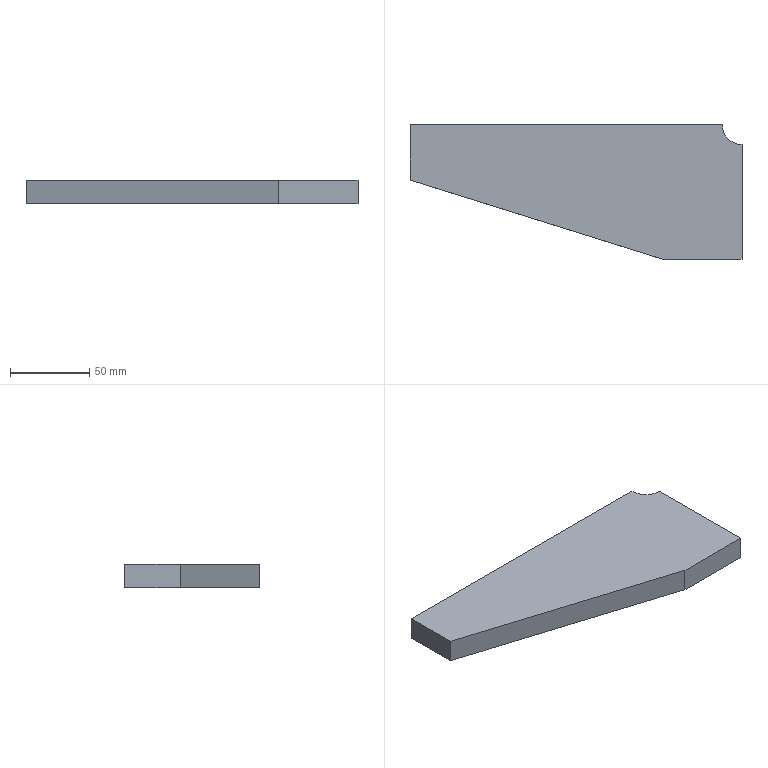Part | STEP file | Input 77 | 1 solid | 8 faces | box 210 x 85 x 15 mm | volume 205909 mm3 | plane 7 | cylinder 1 | commonest cylinder face diameters 25 x1
STEP:
#1=CARTESIAN_POINT('',(0.,0.,0.));
#2=DIRECTION('',(0.,0.,1.));
#3=DIRECTION('',(1.,0.,0.));
#4=AXIS2_PLACEMENT_3D('',#1,#2,#3);
#5=CARTESIAN_POINT('',(4010.,310.,-7.5));
#6=VERTEX_POINT('',#5);
#7=CARTESIAN_POINT('',(3960.,310.,-7.5));
#8=VERTEX_POINT('',#7);
#9=CARTESIAN_POINT('',(3960.,310.,-7.5));
#10=DIRECTION('',(-1.,0.,0.));
#11=VECTOR('',#10,1.);
#12=LINE('',#9,#11);
#13=CARTESIAN_POINT('',(3960.,310.,7.5));
#14=DIRECTION('',(0.,-1.,0.));
#15=DIRECTION('',(-1.,0.,0.));
#16=AXIS2_PLACEMENT_3D('',#13,#14,#15);
#17=PLANE('',#16);
#18=CARTESIAN_POINT('',(0.,15.));
#19=DIRECTION('',(1.,0.));
#20=VECTOR('',#19,1.);
#21=LINE('',#18,#20);
#22=(GEOMETRIC_REPRESENTATION_CONTEXT(2)PARAMETRIC_REPRESENTATION_CONTEXT()REPRESENTATION_CONTEXT('',''));
#23=DEFINITIONAL_REPRESENTATION('',(#21),#22);
#24=PCURVE('',#17,#23);
#25=CARTESIAN_POINT('',(4010.,395.,-7.5));
#26=DIRECTION('',(0.,0.,-1.));
#27=DIRECTION('',(-1.,0.,0.));
#28=AXIS2_PLACEMENT_3D('',#25,#26,#27);
#29=PLANE('',#28);
#30=CARTESIAN_POINT('',(50.,-85.));
#31=DIRECTION('',(1.,0.));
#32=VECTOR('',#31,1.);
#33=LINE('',#30,#32);
#34=(GEOMETRIC_REPRESENTATION_CONTEXT(2)PARAMETRIC_REPRESENTATION_CONTEXT()REPRESENTATION_CONTEXT('',''));
#35=DEFINITIONAL_REPRESENTATION('',(#33),#34);
#36=PCURVE('',#29,#35);
#37=SURFACE_CURVE('',#12,(#24,#36),.PCURVE_S1.);
#38=EDGE_CURVE('',#6,#8,#37,.T.);
#39=ORIENTED_EDGE('',*,*,#38,.F.);
#40=CARTESIAN_POINT('',(4010.,310.,7.5));
#41=VERTEX_POINT('',#40);
#42=CARTESIAN_POINT('',(4010.,310.,7.5));
#43=DIRECTION('',(0.,0.,-1.));
#44=VECTOR('',#43,1.);
#45=LINE('',#42,#44);
#46=CARTESIAN_POINT('',(-50.,0.));
#47=DIRECTION('',(0.,1.));
#48=VECTOR('',#47,1.);
#49=LINE('',#46,#48);
#50=(GEOMETRIC_REPRESENTATION_CONTEXT(2)PARAMETRIC_REPRESENTATION_CONTEXT()REPRESENTATION_CONTEXT('',''));
#51=DEFINITIONAL_REPRESENTATION('',(#49),#50);
#52=PCURVE('',#17,#51);
#53=CARTESIAN_POINT('',(4010.,310.,7.5));
#54=DIRECTION('',(1.,0.,0.));
#55=DIRECTION('',(0.,0.,-1.));
#56=AXIS2_PLACEMENT_3D('',#53,#54,#55);
#57=PLANE('',#56);
#58=CARTESIAN_POINT('',(0.,0.));
#59=DIRECTION('',(1.,0.));
#60=VECTOR('',#59,1.);
#61=LINE('',#58,#60);
#62=(GEOMETRIC_REPRESENTATION_CONTEXT(2)PARAMETRIC_REPRESENTATION_CONTEXT()REPRESENTATION_CONTEXT('',''));
#63=DEFINITIONAL_REPRESENTATION('',(#61),#62);
#64=PCURVE('',#57,#63);
#65=SURFACE_CURVE('',#45,(#52,#64),.PCURVE_S1.);
#66=EDGE_CURVE('',#41,#6,#65,.T.);
#67=ORIENTED_EDGE('',*,*,#66,.F.);
#68=CARTESIAN_POINT('',(3960.,310.,7.5));
#69=VERTEX_POINT('',#68);
#70=CARTESIAN_POINT('',(3960.,310.,7.5));
#71=DIRECTION('',(-1.,0.,0.));
#72=VECTOR('',#71,1.);
#73=LINE('',#70,#72);
#74=CARTESIAN_POINT('',(0.,0.));
#75=DIRECTION('',(1.,0.));
#76=VECTOR('',#75,1.);
#77=LINE('',#74,#76);
#78=(GEOMETRIC_REPRESENTATION_CONTEXT(2)PARAMETRIC_REPRESENTATION_CONTEXT()REPRESENTATION_CONTEXT('',''));
#79=DEFINITIONAL_REPRESENTATION('',(#77),#78);
#80=PCURVE('',#17,#79);
#81=CARTESIAN_POINT('',(4010.,395.,7.5));
#82=DIRECTION('',(0.,0.,-1.));
#83=DIRECTION('',(-1.,0.,0.));
#84=AXIS2_PLACEMENT_3D('',#81,#82,#83);
#85=PLANE('',#84);
#86=CARTESIAN_POINT('',(50.,-85.));
#87=DIRECTION('',(1.,0.));
#88=VECTOR('',#87,1.);
#89=LINE('',#86,#88);
#90=(GEOMETRIC_REPRESENTATION_CONTEXT(2)PARAMETRIC_REPRESENTATION_CONTEXT()REPRESENTATION_CONTEXT('',''));
#91=DEFINITIONAL_REPRESENTATION('',(#89),#90);
#92=PCURVE('',#85,#91);
#93=SURFACE_CURVE('',#73,(#80,#92),.PCURVE_S1.);
#94=EDGE_CURVE('',#41,#69,#93,.T.);
#95=ORIENTED_EDGE('',*,*,#94,.T.);
#96=CARTESIAN_POINT('',(3960.,310.,7.5));
#97=DIRECTION('',(0.,0.,-1.));
#98=VECTOR('',#97,1.);
#99=LINE('',#96,#98);
#100=CARTESIAN_POINT('',(0.,0.));
#101=DIRECTION('',(0.,1.));
#102=VECTOR('',#101,1.);
#103=LINE('',#100,#102);
#104=(GEOMETRIC_REPRESENTATION_CONTEXT(2)PARAMETRIC_REPRESENTATION_CONTEXT()REPRESENTATION_CONTEXT('',''));
#105=DEFINITIONAL_REPRESENTATION('',(#103),#104);
#106=PCURVE('',#17,#105);
#107=CARTESIAN_POINT('',(3800.,360.,7.5));
#108=DIRECTION('',(-0.2983,-0.9545,0.));
#109=DIRECTION('',(-0.9545,0.2983,0.));
#110=AXIS2_PLACEMENT_3D('',#107,#108,#109);
#111=PLANE('',#110);
#112=CARTESIAN_POINT('',(-167.631,0.));
#113=DIRECTION('',(0.,1.));
#114=VECTOR('',#113,1.);
#115=LINE('',#112,#114);
#116=(GEOMETRIC_REPRESENTATION_CONTEXT(2)PARAMETRIC_REPRESENTATION_CONTEXT()REPRESENTATION_CONTEXT('',''));
#117=DEFINITIONAL_REPRESENTATION('',(#115),#116);
#118=PCURVE('',#111,#117);
#119=SURFACE_CURVE('',#99,(#106,#118),.PCURVE_S1.);
#120=EDGE_CURVE('',#69,#8,#119,.T.);
#121=ORIENTED_EDGE('',*,*,#120,.T.);
#122=EDGE_LOOP('',(#39,#67,#95,#121));
#123=FACE_BOUND('',#122,.T.);
#124=ADVANCED_FACE('',(#123),#17,.T.);
#125=CARTESIAN_POINT('',(4010.,382.5,-7.5));
#126=VERTEX_POINT('',#125);
#127=CARTESIAN_POINT('',(4010.,310.,-7.5));
#128=DIRECTION('',(0.,-1.,0.));
#129=VECTOR('',#128,1.);
#130=LINE('',#127,#129);
#131=CARTESIAN_POINT('',(15.,0.));
#132=DIRECTION('',(0.,-1.));
#133=VECTOR('',#132,1.);
#134=LINE('',#131,#133);
#135=(GEOMETRIC_REPRESENTATION_CONTEXT(2)PARAMETRIC_REPRESENTATION_CONTEXT()REPRESENTATION_CONTEXT('',''));
#136=DEFINITIONAL_REPRESENTATION('',(#134),#135);
#137=PCURVE('',#57,#136);
#138=CARTESIAN_POINT('',(0.,-85.));
#139=DIRECTION('',(0.,-1.));
#140=VECTOR('',#139,1.);
#141=LINE('',#138,#140);
#142=(GEOMETRIC_REPRESENTATION_CONTEXT(2)PARAMETRIC_REPRESENTATION_CONTEXT()REPRESENTATION_CONTEXT('',''));
#143=DEFINITIONAL_REPRESENTATION('',(#141),#142);
#144=PCURVE('',#29,#143);
#145=SURFACE_CURVE('',#130,(#137,#144),.PCURVE_S1.);
#146=EDGE_CURVE('',#126,#6,#145,.T.);
#147=ORIENTED_EDGE('',*,*,#146,.F.);
#148=CARTESIAN_POINT('',(4010.,382.5,7.5));
#149=VERTEX_POINT('',#148);
#150=CARTESIAN_POINT('',(4010.,382.5,7.5));
#151=DIRECTION('',(0.,0.,-1.));
#152=VECTOR('',#151,1.);
#153=LINE('',#150,#152);
#154=CARTESIAN_POINT('',(0.,72.5));
#155=DIRECTION('',(1.,0.));
#156=VECTOR('',#155,1.);
#157=LINE('',#154,#156);
#158=(GEOMETRIC_REPRESENTATION_CONTEXT(2)PARAMETRIC_REPRESENTATION_CONTEXT()REPRESENTATION_CONTEXT('',''));
#159=DEFINITIONAL_REPRESENTATION('',(#157),#158);
#160=PCURVE('',#57,#159);
#161=CARTESIAN_POINT('',(4010.,395.,7.5));
#162=DIRECTION('',(0.,0.,-1.));
#163=DIRECTION('',(-1.,0.,0.));
#164=AXIS2_PLACEMENT_3D('',#161,#162,#163);
#165=CYLINDRICAL_SURFACE('',#164,12.5);
#166=CARTESIAN_POINT('',(4.712,0.));
#167=DIRECTION('',(0.,1.));
#168=VECTOR('',#167,1.);
#169=LINE('',#166,#168);
#170=(GEOMETRIC_REPRESENTATION_CONTEXT(2)PARAMETRIC_REPRESENTATION_CONTEXT()REPRESENTATION_CONTEXT('',''));
#171=DEFINITIONAL_REPRESENTATION('',(#169),#170);
#172=PCURVE('',#165,#171);
#173=SURFACE_CURVE('',#153,(#160,#172),.PCURVE_S1.);
#174=EDGE_CURVE('',#149,#126,#173,.T.);
#175=ORIENTED_EDGE('',*,*,#174,.F.);
#176=CARTESIAN_POINT('',(4010.,310.,7.5));
#177=DIRECTION('',(0.,-1.,0.));
#178=VECTOR('',#177,1.);
#179=LINE('',#176,#178);
#180=CARTESIAN_POINT('',(0.,0.));
#181=DIRECTION('',(0.,-1.));
#182=VECTOR('',#181,1.);
#183=LINE('',#180,#182);
#184=(GEOMETRIC_REPRESENTATION_CONTEXT(2)PARAMETRIC_REPRESENTATION_CONTEXT()REPRESENTATION_CONTEXT('',''));
#185=DEFINITIONAL_REPRESENTATION('',(#183),#184);
#186=PCURVE('',#57,#185);
#187=CARTESIAN_POINT('',(0.,-85.));
#188=DIRECTION('',(0.,-1.));
#189=VECTOR('',#188,1.);
#190=LINE('',#187,#189);
#191=(GEOMETRIC_REPRESENTATION_CONTEXT(2)PARAMETRIC_REPRESENTATION_CONTEXT()REPRESENTATION_CONTEXT('',''));
#192=DEFINITIONAL_REPRESENTATION('',(#190),#191);
#193=PCURVE('',#85,#192);
#194=SURFACE_CURVE('',#179,(#186,#193),.PCURVE_S1.);
#195=EDGE_CURVE('',#149,#41,#194,.T.);
#196=ORIENTED_EDGE('',*,*,#195,.T.);
#197=ORIENTED_EDGE('',*,*,#66,.T.);
#198=EDGE_LOOP('',(#147,#175,#196,#197));
#199=FACE_BOUND('',#198,.T.);
#200=ADVANCED_FACE('',(#199),#57,.T.);
#201=ORIENTED_EDGE('',*,*,#174,.F.);
#202=CARTESIAN_POINT('',(3997.5,395.,7.5));
#203=VERTEX_POINT('',#202);
#204=CARTESIAN_POINT('',(4010.,395.,7.5));
#205=DIRECTION('',(0.,0.,1.));
#206=DIRECTION('',(-1.,0.,0.));
#207=AXIS2_PLACEMENT_3D('',#204,#205,#206);
#208=CIRCLE('',#207,12.5);
#209=CARTESIAN_POINT('',(6.283,0.));
#210=DIRECTION('',(-1.,0.));
#211=VECTOR('',#210,1.);
#212=LINE('',#209,#211);
#213=(GEOMETRIC_REPRESENTATION_CONTEXT(2)PARAMETRIC_REPRESENTATION_CONTEXT()REPRESENTATION_CONTEXT('',''));
#214=DEFINITIONAL_REPRESENTATION('',(#212),#213);
#215=PCURVE('',#165,#214);
#216=CARTESIAN_POINT('',(12.5,0.));
#217=CARTESIAN_POINT('',(12.5,-21.651));
#218=CARTESIAN_POINT('',(-6.25,-10.825));
#219=CARTESIAN_POINT('',(-25.,0.));
#220=CARTESIAN_POINT('',(-6.25,10.825));
#221=CARTESIAN_POINT('',(12.5,21.651));
#222=CARTESIAN_POINT('',(12.5,0.));
#223=(BOUNDED_CURVE()B_SPLINE_CURVE(2,(#216,#217,#218,#219,#220,#221,#222),.UNSPECIFIED.,.T.,.F.)B_SPLINE_CURVE_WITH_KNOTS((1,2,2,2,2,1),(-2.094,0.,2.094,4.189,6.283,8.378),.UNSPECIFIED.)CURVE()GEOMETRIC_REPRESENTATION_ITEM()RATIONAL_B_SPLINE_CURVE((1.,0.5,1.,0.5,1.,0.5,1.))REPRESENTATION_ITEM(''));
#224=(GEOMETRIC_REPRESENTATION_CONTEXT(2)PARAMETRIC_REPRESENTATION_CONTEXT()REPRESENTATION_CONTEXT('',''));
#225=DEFINITIONAL_REPRESENTATION('',(#223),#224);
#226=PCURVE('',#85,#225);
#227=SURFACE_CURVE('',#208,(#215,#226),.PCURVE_S1.);
#228=EDGE_CURVE('',#203,#149,#227,.T.);
#229=ORIENTED_EDGE('',*,*,#228,.F.);
#230=CARTESIAN_POINT('',(3997.5,395.,-7.5));
#231=VERTEX_POINT('',#230);
#232=CARTESIAN_POINT('',(3997.5,395.,7.5));
#233=DIRECTION('',(0.,0.,-1.));
#234=VECTOR('',#233,1.);
#235=LINE('',#232,#234);
#236=CARTESIAN_POINT('',(6.283,0.));
#237=DIRECTION('',(0.,1.));
#238=VECTOR('',#237,1.);
#239=LINE('',#236,#238);
#240=(GEOMETRIC_REPRESENTATION_CONTEXT(2)PARAMETRIC_REPRESENTATION_CONTEXT()REPRESENTATION_CONTEXT('',''));
#241=DEFINITIONAL_REPRESENTATION('',(#239),#240);
#242=PCURVE('',#165,#241);
#243=CARTESIAN_POINT('',(3997.5,395.,7.5));
#244=DIRECTION('',(0.,1.,0.));
#245=DIRECTION('',(0.,0.,-1.));
#246=AXIS2_PLACEMENT_3D('',#243,#244,#245);
#247=PLANE('',#246);
#248=CARTESIAN_POINT('',(0.,0.));
#249=DIRECTION('',(1.,0.));
#250=VECTOR('',#249,1.);
#251=LINE('',#248,#250);
#252=(GEOMETRIC_REPRESENTATION_CONTEXT(2)PARAMETRIC_REPRESENTATION_CONTEXT()REPRESENTATION_CONTEXT('',''));
#253=DEFINITIONAL_REPRESENTATION('',(#251),#252);
#254=PCURVE('',#247,#253);
#255=SURFACE_CURVE('',#235,(#242,#254),.PCURVE_S1.);
#256=EDGE_CURVE('',#203,#231,#255,.T.);
#257=ORIENTED_EDGE('',*,*,#256,.T.);
#258=CARTESIAN_POINT('',(4010.,395.,-7.5));
#259=DIRECTION('',(0.,0.,1.));
#260=DIRECTION('',(-1.,0.,0.));
#261=AXIS2_PLACEMENT_3D('',#258,#259,#260);
#262=CIRCLE('',#261,12.5);
#263=CARTESIAN_POINT('',(6.283,15.));
#264=DIRECTION('',(-1.,0.));
#265=VECTOR('',#264,1.);
#266=LINE('',#263,#265);
#267=(GEOMETRIC_REPRESENTATION_CONTEXT(2)PARAMETRIC_REPRESENTATION_CONTEXT()REPRESENTATION_CONTEXT('',''));
#268=DEFINITIONAL_REPRESENTATION('',(#266),#267);
#269=PCURVE('',#165,#268);
#270=CARTESIAN_POINT('',(12.5,0.));
#271=CARTESIAN_POINT('',(12.5,-21.651));
#272=CARTESIAN_POINT('',(-6.25,-10.825));
#273=CARTESIAN_POINT('',(-25.,0.));
#274=CARTESIAN_POINT('',(-6.25,10.825));
#275=CARTESIAN_POINT('',(12.5,21.651));
#276=CARTESIAN_POINT('',(12.5,0.));
#277=(BOUNDED_CURVE()B_SPLINE_CURVE(2,(#270,#271,#272,#273,#274,#275,#276),.UNSPECIFIED.,.T.,.F.)B_SPLINE_CURVE_WITH_KNOTS((1,2,2,2,2,1),(-2.094,0.,2.094,4.189,6.283,8.378),.UNSPECIFIED.)CURVE()GEOMETRIC_REPRESENTATION_ITEM()RATIONAL_B_SPLINE_CURVE((1.,0.5,1.,0.5,1.,0.5,1.))REPRESENTATION_ITEM(''));
#278=(GEOMETRIC_REPRESENTATION_CONTEXT(2)PARAMETRIC_REPRESENTATION_CONTEXT()REPRESENTATION_CONTEXT('',''));
#279=DEFINITIONAL_REPRESENTATION('',(#277),#278);
#280=PCURVE('',#29,#279);
#281=SURFACE_CURVE('',#262,(#269,#280),.PCURVE_S1.);
#282=EDGE_CURVE('',#231,#126,#281,.T.);
#283=ORIENTED_EDGE('',*,*,#282,.T.);
#284=EDGE_LOOP('',(#201,#229,#257,#283));
#285=FACE_BOUND('',#284,.F.);
#286=ADVANCED_FACE('',(#285),#165,.F.);
#287=CARTESIAN_POINT('',(3800.,395.,-7.5));
#288=VERTEX_POINT('',#287);
#289=CARTESIAN_POINT('',(3997.5,395.,-7.5));
#290=DIRECTION('',(1.,0.,0.));
#291=VECTOR('',#290,1.);
#292=LINE('',#289,#291);
#293=CARTESIAN_POINT('',(15.,0.));
#294=DIRECTION('',(0.,-1.));
#295=VECTOR('',#294,1.);
#296=LINE('',#293,#295);
#297=(GEOMETRIC_REPRESENTATION_CONTEXT(2)PARAMETRIC_REPRESENTATION_CONTEXT()REPRESENTATION_CONTEXT('',''));
#298=DEFINITIONAL_REPRESENTATION('',(#296),#297);
#299=PCURVE('',#247,#298);
#300=CARTESIAN_POINT('',(12.5,0.));
#301=DIRECTION('',(-1.,0.));
#302=VECTOR('',#301,1.);
#303=LINE('',#300,#302);
#304=(GEOMETRIC_REPRESENTATION_CONTEXT(2)PARAMETRIC_REPRESENTATION_CONTEXT()REPRESENTATION_CONTEXT('',''));
#305=DEFINITIONAL_REPRESENTATION('',(#303),#304);
#306=PCURVE('',#29,#305);
#307=SURFACE_CURVE('',#292,(#299,#306),.PCURVE_S1.);
#308=EDGE_CURVE('',#288,#231,#307,.T.);
#309=ORIENTED_EDGE('',*,*,#308,.F.);
#310=CARTESIAN_POINT('',(3800.,395.,7.5));
#311=VERTEX_POINT('',#310);
#312=CARTESIAN_POINT('',(3800.,395.,7.5));
#313=DIRECTION('',(0.,0.,-1.));
#314=VECTOR('',#313,1.);
#315=LINE('',#312,#314);
#316=CARTESIAN_POINT('',(0.,197.5));
#317=DIRECTION('',(1.,0.));
#318=VECTOR('',#317,1.);
#319=LINE('',#316,#318);
#320=(GEOMETRIC_REPRESENTATION_CONTEXT(2)PARAMETRIC_REPRESENTATION_CONTEXT()REPRESENTATION_CONTEXT('',''));
#321=DEFINITIONAL_REPRESENTATION('',(#319),#320);
#322=PCURVE('',#247,#321);
#323=CARTESIAN_POINT('',(3800.,395.,7.5));
#324=DIRECTION('',(-1.,0.,0.));
#325=DIRECTION('',(0.,1.,0.));
#326=AXIS2_PLACEMENT_3D('',#323,#324,#325);
#327=PLANE('',#326);
#328=CARTESIAN_POINT('',(0.,0.));
#329=DIRECTION('',(0.,1.));
#330=VECTOR('',#329,1.);
#331=LINE('',#328,#330);
#332=(GEOMETRIC_REPRESENTATION_CONTEXT(2)PARAMETRIC_REPRESENTATION_CONTEXT()REPRESENTATION_CONTEXT('',''));
#333=DEFINITIONAL_REPRESENTATION('',(#331),#332);
#334=PCURVE('',#327,#333);
#335=SURFACE_CURVE('',#315,(#322,#334),.PCURVE_S1.);
#336=EDGE_CURVE('',#311,#288,#335,.T.);
#337=ORIENTED_EDGE('',*,*,#336,.F.);
#338=CARTESIAN_POINT('',(3997.5,395.,7.5));
#339=DIRECTION('',(1.,0.,0.));
#340=VECTOR('',#339,1.);
#341=LINE('',#338,#340);
#342=CARTESIAN_POINT('',(0.,0.));
#343=DIRECTION('',(0.,-1.));
#344=VECTOR('',#343,1.);
#345=LINE('',#342,#344);
#346=(GEOMETRIC_REPRESENTATION_CONTEXT(2)PARAMETRIC_REPRESENTATION_CONTEXT()REPRESENTATION_CONTEXT('',''));
#347=DEFINITIONAL_REPRESENTATION('',(#345),#346);
#348=PCURVE('',#247,#347);
#349=CARTESIAN_POINT('',(12.5,0.));
#350=DIRECTION('',(-1.,0.));
#351=VECTOR('',#350,1.);
#352=LINE('',#349,#351);
#353=(GEOMETRIC_REPRESENTATION_CONTEXT(2)PARAMETRIC_REPRESENTATION_CONTEXT()REPRESENTATION_CONTEXT('',''));
#354=DEFINITIONAL_REPRESENTATION('',(#352),#353);
#355=PCURVE('',#85,#354);
#356=SURFACE_CURVE('',#341,(#348,#355),.PCURVE_S1.);
#357=EDGE_CURVE('',#311,#203,#356,.T.);
#358=ORIENTED_EDGE('',*,*,#357,.T.);
#359=ORIENTED_EDGE('',*,*,#256,.T.);
#360=EDGE_LOOP('',(#309,#337,#358,#359));
#361=FACE_BOUND('',#360,.T.);
#362=ADVANCED_FACE('',(#361),#247,.T.);
#363=CARTESIAN_POINT('',(3800.,360.,-7.5));
#364=VERTEX_POINT('',#363);
#365=CARTESIAN_POINT('',(3800.,395.,-7.5));
#366=DIRECTION('',(0.,1.,0.));
#367=VECTOR('',#366,1.);
#368=LINE('',#365,#367);
#369=CARTESIAN_POINT('',(0.,15.));
#370=DIRECTION('',(1.,0.));
#371=VECTOR('',#370,1.);
#372=LINE('',#369,#371);
#373=(GEOMETRIC_REPRESENTATION_CONTEXT(2)PARAMETRIC_REPRESENTATION_CONTEXT()REPRESENTATION_CONTEXT('',''));
#374=DEFINITIONAL_REPRESENTATION('',(#372),#373);
#375=PCURVE('',#327,#374);
#376=CARTESIAN_POINT('',(210.,0.));
#377=DIRECTION('',(0.,1.));
#378=VECTOR('',#377,1.);
#379=LINE('',#376,#378);
#380=(GEOMETRIC_REPRESENTATION_CONTEXT(2)PARAMETRIC_REPRESENTATION_CONTEXT()REPRESENTATION_CONTEXT('',''));
#381=DEFINITIONAL_REPRESENTATION('',(#379),#380);
#382=PCURVE('',#29,#381);
#383=SURFACE_CURVE('',#368,(#375,#382),.PCURVE_S1.);
#384=EDGE_CURVE('',#364,#288,#383,.T.);
#385=ORIENTED_EDGE('',*,*,#384,.F.);
#386=CARTESIAN_POINT('',(3800.,360.,7.5));
#387=VERTEX_POINT('',#386);
#388=CARTESIAN_POINT('',(3800.,360.,7.5));
#389=DIRECTION('',(0.,0.,-1.));
#390=VECTOR('',#389,1.);
#391=LINE('',#388,#390);
#392=CARTESIAN_POINT('',(-35.,0.));
#393=DIRECTION('',(0.,1.));
#394=VECTOR('',#393,1.);
#395=LINE('',#392,#394);
#396=(GEOMETRIC_REPRESENTATION_CONTEXT(2)PARAMETRIC_REPRESENTATION_CONTEXT()REPRESENTATION_CONTEXT('',''));
#397=DEFINITIONAL_REPRESENTATION('',(#395),#396);
#398=PCURVE('',#327,#397);
#399=CARTESIAN_POINT('',(0.,0.));
#400=DIRECTION('',(0.,1.));
#401=VECTOR('',#400,1.);
#402=LINE('',#399,#401);
#403=(GEOMETRIC_REPRESENTATION_CONTEXT(2)PARAMETRIC_REPRESENTATION_CONTEXT()REPRESENTATION_CONTEXT('',''));
#404=DEFINITIONAL_REPRESENTATION('',(#402),#403);
#405=PCURVE('',#111,#404);
#406=SURFACE_CURVE('',#391,(#398,#405),.PCURVE_S1.);
#407=EDGE_CURVE('',#387,#364,#406,.T.);
#408=ORIENTED_EDGE('',*,*,#407,.F.);
#409=CARTESIAN_POINT('',(3800.,395.,7.5));
#410=DIRECTION('',(0.,1.,0.));
#411=VECTOR('',#410,1.);
#412=LINE('',#409,#411);
#413=CARTESIAN_POINT('',(0.,0.));
#414=DIRECTION('',(1.,0.));
#415=VECTOR('',#414,1.);
#416=LINE('',#413,#415);
#417=(GEOMETRIC_REPRESENTATION_CONTEXT(2)PARAMETRIC_REPRESENTATION_CONTEXT()REPRESENTATION_CONTEXT('',''));
#418=DEFINITIONAL_REPRESENTATION('',(#416),#417);
#419=PCURVE('',#327,#418);
#420=CARTESIAN_POINT('',(210.,0.));
#421=DIRECTION('',(0.,1.));
#422=VECTOR('',#421,1.);
#423=LINE('',#420,#422);
#424=(GEOMETRIC_REPRESENTATION_CONTEXT(2)PARAMETRIC_REPRESENTATION_CONTEXT()REPRESENTATION_CONTEXT('',''));
#425=DEFINITIONAL_REPRESENTATION('',(#423),#424);
#426=PCURVE('',#85,#425);
#427=SURFACE_CURVE('',#412,(#419,#426),.PCURVE_S1.);
#428=EDGE_CURVE('',#387,#311,#427,.T.);
#429=ORIENTED_EDGE('',*,*,#428,.T.);
#430=ORIENTED_EDGE('',*,*,#336,.T.);
#431=EDGE_LOOP('',(#385,#408,#429,#430));
#432=FACE_BOUND('',#431,.T.);
#433=ADVANCED_FACE('',(#432),#327,.T.);
#434=CARTESIAN_POINT('',(3800.,360.,-7.5));
#435=DIRECTION('',(-0.9545,0.2983,0.));
#436=VECTOR('',#435,1.);
#437=LINE('',#434,#436);
#438=CARTESIAN_POINT('',(0.,15.));
#439=DIRECTION('',(1.,0.));
#440=VECTOR('',#439,1.);
#441=LINE('',#438,#440);
#442=(GEOMETRIC_REPRESENTATION_CONTEXT(2)PARAMETRIC_REPRESENTATION_CONTEXT()REPRESENTATION_CONTEXT('',''));
#443=DEFINITIONAL_REPRESENTATION('',(#441),#442);
#444=PCURVE('',#111,#443);
#445=CARTESIAN_POINT('',(210.,-35.));
#446=DIRECTION('',(0.9545,0.2983));
#447=VECTOR('',#446,1.);
#448=LINE('',#445,#447);
#449=(GEOMETRIC_REPRESENTATION_CONTEXT(2)PARAMETRIC_REPRESENTATION_CONTEXT()REPRESENTATION_CONTEXT('',''));
#450=DEFINITIONAL_REPRESENTATION('',(#448),#449);
#451=PCURVE('',#29,#450);
#452=SURFACE_CURVE('',#437,(#444,#451),.PCURVE_S1.);
#453=EDGE_CURVE('',#8,#364,#452,.T.);
#454=ORIENTED_EDGE('',*,*,#453,.F.);
#455=ORIENTED_EDGE('',*,*,#120,.F.);
#456=CARTESIAN_POINT('',(3800.,360.,7.5));
#457=DIRECTION('',(-0.9545,0.2983,0.));
#458=VECTOR('',#457,1.);
#459=LINE('',#456,#458);
#460=CARTESIAN_POINT('',(0.,0.));
#461=DIRECTION('',(1.,0.));
#462=VECTOR('',#461,1.);
#463=LINE('',#460,#462);
#464=(GEOMETRIC_REPRESENTATION_CONTEXT(2)PARAMETRIC_REPRESENTATION_CONTEXT()REPRESENTATION_CONTEXT('',''));
#465=DEFINITIONAL_REPRESENTATION('',(#463),#464);
#466=PCURVE('',#111,#465);
#467=CARTESIAN_POINT('',(210.,-35.));
#468=DIRECTION('',(0.9545,0.2983));
#469=VECTOR('',#468,1.);
#470=LINE('',#467,#469);
#471=(GEOMETRIC_REPRESENTATION_CONTEXT(2)PARAMETRIC_REPRESENTATION_CONTEXT()REPRESENTATION_CONTEXT('',''));
#472=DEFINITIONAL_REPRESENTATION('',(#470),#471);
#473=PCURVE('',#85,#472);
#474=SURFACE_CURVE('',#459,(#466,#473),.PCURVE_S1.);
#475=EDGE_CURVE('',#69,#387,#474,.T.);
#476=ORIENTED_EDGE('',*,*,#475,.T.);
#477=ORIENTED_EDGE('',*,*,#407,.T.);
#478=EDGE_LOOP('',(#454,#455,#476,#477));
#479=FACE_BOUND('',#478,.T.);
#480=ADVANCED_FACE('',(#479),#111,.T.);
#481=ORIENTED_EDGE('',*,*,#94,.F.);
#482=ORIENTED_EDGE('',*,*,#195,.F.);
#483=ORIENTED_EDGE('',*,*,#228,.F.);
#484=ORIENTED_EDGE('',*,*,#357,.F.);
#485=ORIENTED_EDGE('',*,*,#428,.F.);
#486=ORIENTED_EDGE('',*,*,#475,.F.);
#487=EDGE_LOOP('',(#481,#482,#483,#484,#485,#486));
#488=FACE_BOUND('',#487,.T.);
#489=ADVANCED_FACE('',(#488),#85,.F.);
#490=ORIENTED_EDGE('',*,*,#38,.T.);
#491=ORIENTED_EDGE('',*,*,#453,.T.);
#492=ORIENTED_EDGE('',*,*,#384,.T.);
#493=ORIENTED_EDGE('',*,*,#308,.T.);
#494=ORIENTED_EDGE('',*,*,#282,.T.);
#495=ORIENTED_EDGE('',*,*,#146,.T.);
#496=EDGE_LOOP('',(#490,#491,#492,#493,#494,#495));
#497=FACE_BOUND('',#496,.T.);
#498=ADVANCED_FACE('',(#497),#29,.T.);
#499=CLOSED_SHELL('',(#124,#200,#286,#362,#433,#480,#489,#498));
#500=MANIFOLD_SOLID_BREP('',#499);
#501=(LENGTH_UNIT()NAMED_UNIT(*)SI_UNIT(.MILLI.,.METRE.));
#502=UNCERTAINTY_MEASURE_WITH_UNIT(LENGTH_MEASURE(0.0000001),#501,'','');
#503=(NAMED_UNIT(*)PLANE_ANGLE_UNIT()SI_UNIT($,.RADIAN.));
#504=(NAMED_UNIT(*)SI_UNIT($,.STERADIAN.)SOLID_ANGLE_UNIT());
#505=(GEOMETRIC_REPRESENTATION_CONTEXT(3)GLOBAL_UNCERTAINTY_ASSIGNED_CONTEXT((#502))GLOBAL_UNIT_ASSIGNED_CONTEXT((#501,#503,#504))REPRESENTATION_CONTEXT('',''));
#506=ADVANCED_BREP_SHAPE_REPRESENTATION('',(#4,#500),#505);